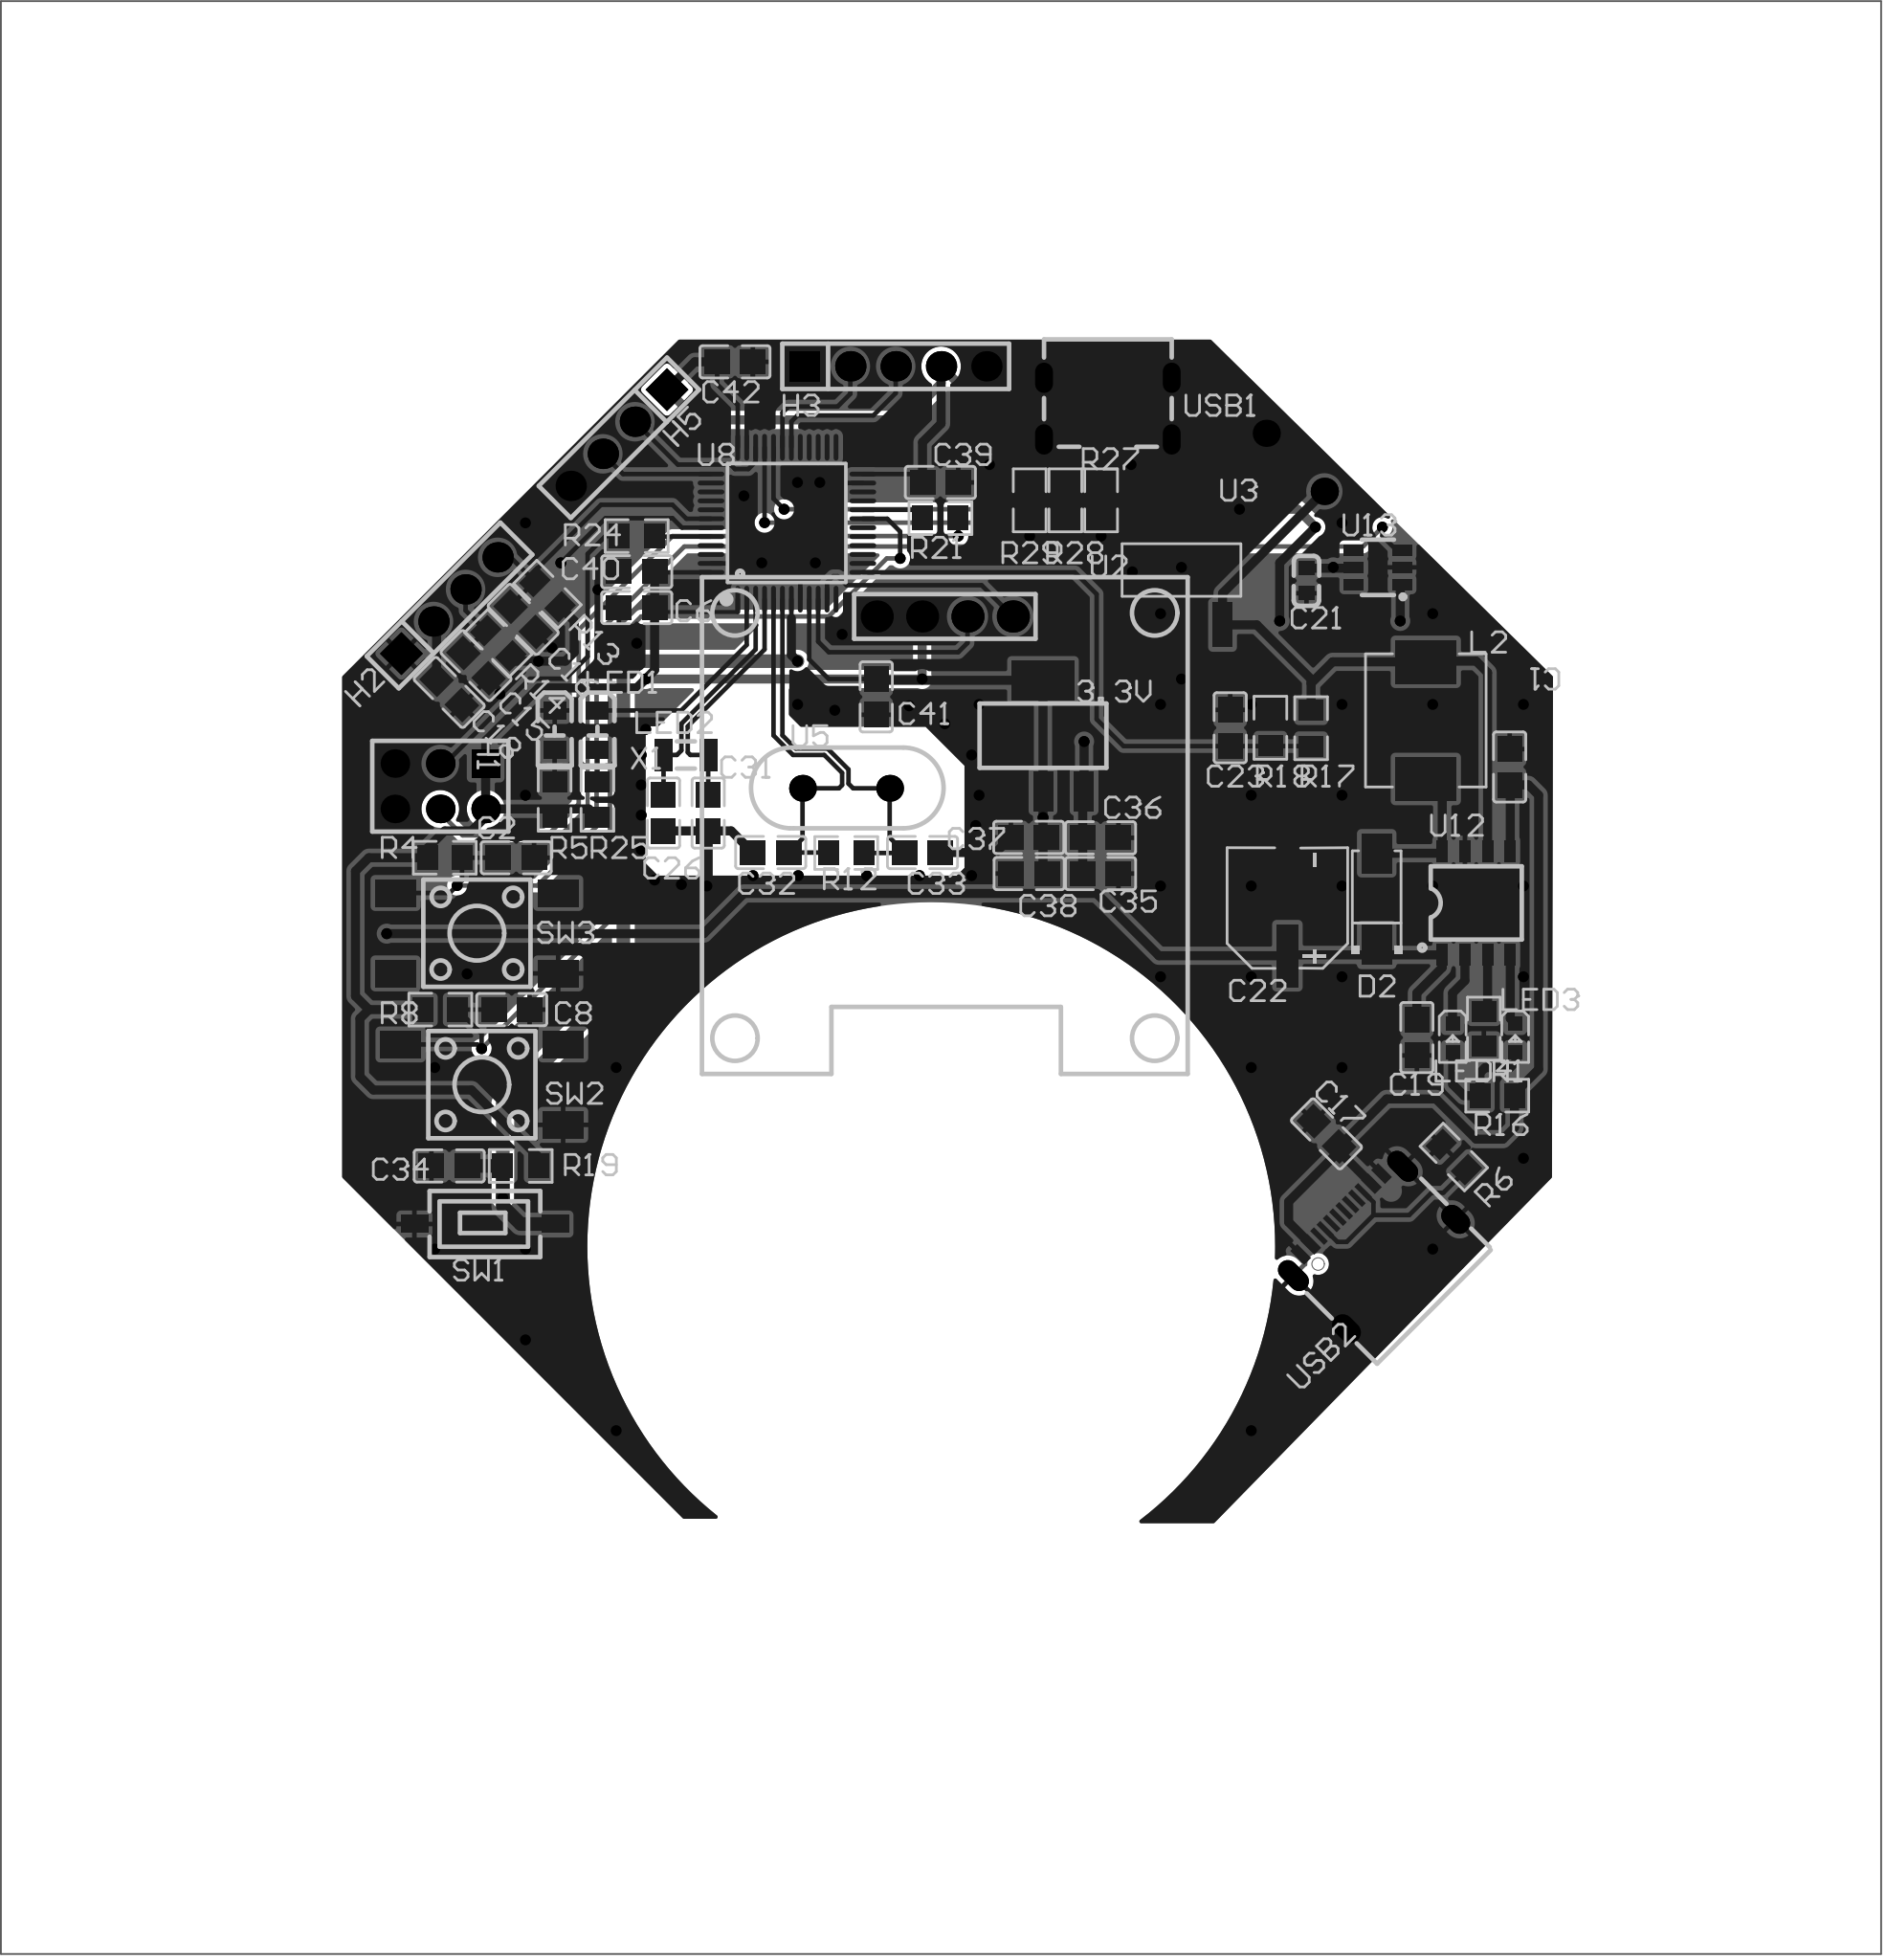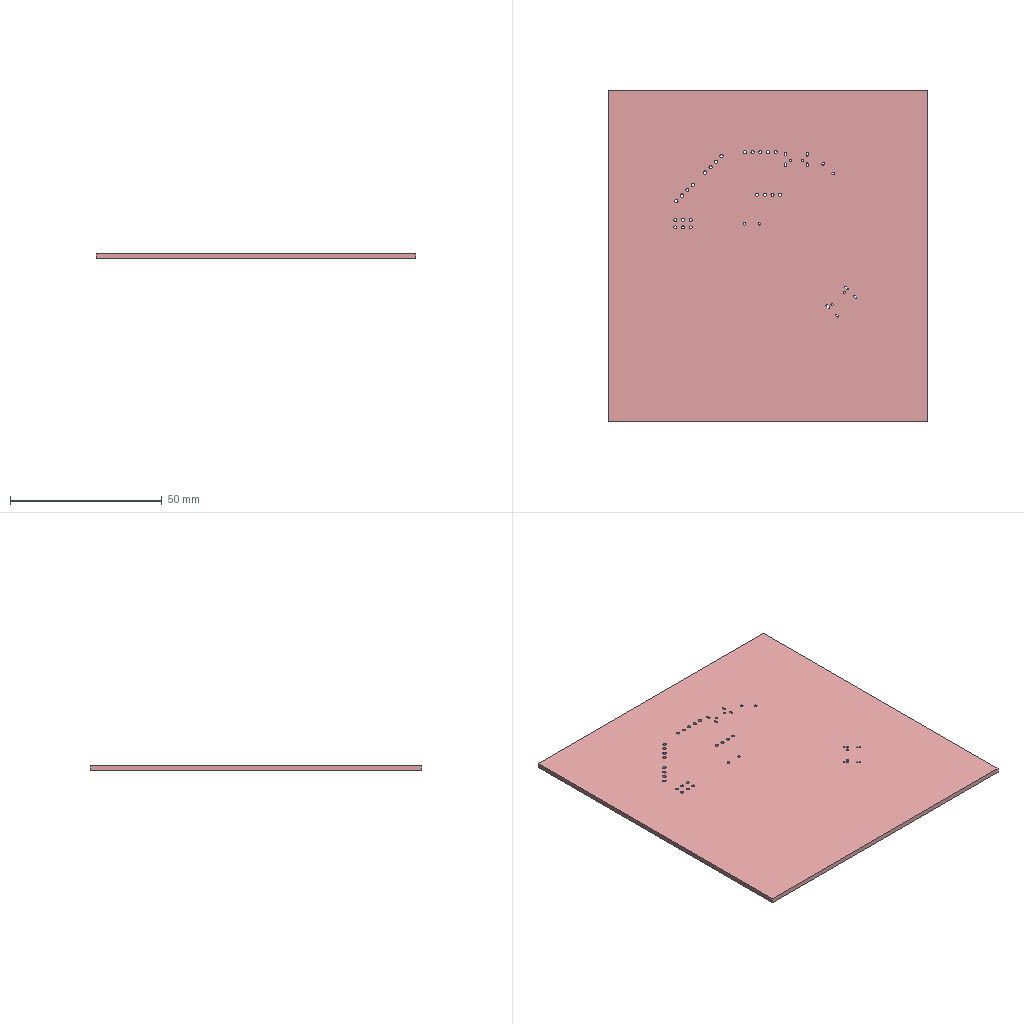Circuit board layout | Altium Designer | box 105.3 x 109.3 x 1.6 mm
Layer stack:
# Altium Designer layer stack of  (unit mm; dielectric type: 0 none, 1 core, 2 prepreg, 3 surface material)
index,name,kind,layer,copper_thickness_mm,dielectric_type,dielectric_thickness_mm,dielectric_material,dielectric_constant
0,Top Paste Mask Layer,other,,,,,,
1,Top Silkscreen Layer,other,,,,,,
2,Top Solder Mask Layer,dielectric,,,3,0.01,,3.3
3,Top Layer,copper,Top Layer,0.035,,,,
4,Dielectric1,dielectric,,,3,1.51,FR4,4.5
5,Bottom Layer,copper,Bottom Layer,0.035,,,,
6,Bottom Solder Mask Layer,dielectric,,,3,0.01,,3.3
7,Bottom Silkscreen Layer,other,,,,,,
8,Bottom Paste Mask Layer,other,,,,,,
# drill layer pairs: low layer,high layer
drill_pair,Top Layer,Bottom Layer
Part placement:
Designator,Comment,Layer,Footprint,Center-X(mm),Center-Y(mm),Rotation
R1,10Ω,TopLayer,R0805_NEW,152.883,121.634,90
C2,0.1uF,TopLayer,C0805,98.703,131.2,0
R12,1M,TopLayer,R0805,117.181,131.464,180
USB1,,TopLayer,USB_Micro,131.832,156.333,180
C8,0.1uF,TopLayer,C0805,98.453,122.7,0
C37,10UF,TopLayer,C0805,127.401,132.338,0
R21,10K,TopLayer,R0805,122.457,150.2,180
R25,510R,TopLayer,R0805,103.252,134.445,90
R28,20R,TopLayer,R0805,129.452,151.2,270
C38,100nF,TopLayer,C0805,127.422,130.314,0
C39,100nF,TopLayer,C0805,122.453,152.2,180
C15,0.1uF,TopLayer,C0805,96.453,141.95,135
C40,100nF,TopLayer,C0805,105.453,147.2,0
C16,0.1uF,TopLayer,C0805,99.095,144.539,135
C17,0.1uF,TopLayer,C0805,144.07,115.746,315
C18,0.1uF,TopLayer,C0805,94.953,140.45,315
C41,100nF,TopLayer,C0805,118.861,140.2,90
C19,100nF,TopLayer,C0805,149.133,121.134,270
C42,100nF,TopLayer,C0805,110.953,158.95,180
C21,100nF,TopLayer,C0603,142.952,146.7,90
C1,10uF,TopLayer,C0805,154.329,136.277,270
C22,47uF,TopLayer,CAP-SMD_BD6.3-L6.6-W6.6-LS7.2-FD,141.884,128.384,90
C23,100nF,TopLayer,C0805,138.681,138.471,90
H1,,TopLayer,HDR-TH_6P-P2.54-V-R2-C3-S2.54_A2541WV-2X3P,94.453,135.2,180
D2,SS14,TopLayer,SMA_L4.2-W2.6-LS5.3-RD,146.883,128.884,90
R19,10K,TopLayer,R0805,98.953,113.95,0
H2,2.54-1*4P排针母座,TopLayer,HDR-TH_4P-P2.54-V-F,94.97,145.316,45
H3,PZ254-1-05-Z-8.5,TopLayer,HDR-TH_5P-P2.54-V-M,119.953,158.7,0
R27,20R,TopLayer,R0805,131.452,151.2,270
SW1,,TopLayer,Key_SMD_3.6x6.1x2.5,96.953,110.7,0
L2,10uH,TopLayer,IND-SMD_L7.3-W6.6,149.633,138.884,270
C32,20PF,TopLayer,C0805,112.953,131.489,180
C33,20PF,TopLayer,C0805,121.453,131.489,0
U5,8MHz,TopLayer,CRYSTAL-TH_L10.8-W4.5-P4.88,117.174,135.085,180
R4,10K,TopLayer,R0805_NEW,94.703,131.2,180
R6,5.1kΩ,TopLayer,R0805,151.202,114.45,135
LED2,,TopLayer,LED_0805,103.257,138.341,270
R8,10K,TopLayer,R0805_NEW,94.453,122.7,180
C6,100nF,TopLayer,C0805,105.453,145.2,0
3.3V,,TopLayer,SOT_223,128.201,138.029,0
C36,100nF,TopLayer,C0805,131.423,132.314,180
R5,510R,TopLayer,R0805,100.853,134.445,90
R13,1kΩ,TopLayer,R0805,100.453,145.95,315
C35,1UF,TopLayer,C0805,131.423,130.314,180
R14,1kΩ,TopLayer,R0805,97.703,143.2,315
C31,20PF,TopLayer,C0805,109.453,133.7,90
R16,2K,TopLayer,R0805_NEW,153.633,117.884,0
LED3,NCD0603R1,TopLayer,LED0603-RD_RED,154.633,121.134,270
R17,100kΩ,TopLayer,R0805,143.21,138.446,270
LED4,NCD0603R1,TopLayer,LED0603-RD_RED,151.133,121.134,270
R18,100kΩ,TopLayer,R0805,140.931,138.471,90
SW2,TS-1002S-13026C,TopLayer,SW-SMD_4P-L6.0-W6.0-P4.50-LS9.0-2,96.78,118.5,0
SW3,TS-1002S-13026C,TopLayer,SW-SMD_4P-L6.0-W6.0-P4.50-LS9.0-2,96.503,126.976,0
LED1,,TopLayer,LED_0805,100.858,138.341,270
H5,,TopLayer,HDR-TH_4P-P2.54-V-M,104.453,154.7,225
R29,5.1K,TopLayer,R0805,127.453,151.2,270
U3,AMS1117-3.3,TopLayer,SOT-223-3_L6.5-W3.5-P3.05-LS7.0,135.952,147.2,270
R24,10K,TopLayer,R0805,105.448,149.2,180
C34,105,0603,TopLayer,C0805,94.953,113.95,0
U8,STM32F103C8T6,TopLayer,LQFP-48_L7.0-W7.0-P0.50-LS9.0-BL,113.86,149.919,0
USB2,TYPE-C 16PIN 2MD(073),TopLayer,USB-C-SMD_TYPE-C-6PIN-2MD-073,146.765,109.388,45
X1,32.768kHz,TopLayer,FC-135R_L3.2-W1.5,108.203,136.95,180
U12,TP5400,TopLayer,ESOP-8_L4.9-W3.9-P1.27-LS6.0-BL-EP,152.459,128.669,0
C26,20PF,TopLayer,C0805,106.953,133.7,270
U13,EC190708,TopLayer,SOT-23-6_L2.9-W1.6-P0.95-LS2.8-BR,146.952,147.45,0
U2,HS96L03W2C03,TopLayer,OLED-TH_L27.8-W27.2-P2.54_C9900033791,122.703,144.7,0
Pad and via stacks:
# Altium Designer via and pad stacks of  (unit mm). Each distinct definition once, with the count of objects using it.
# via: kind,start_layer,end_layer,hole_mm,diameter_mm,mode(0 simple;1 top-mid-bottom;2 full stack),diameter_per_layer,count,example_net
# pad: kind,layer,hole_mm,hole_type(0 round;1 square;2 slot),plating,top_size,top_shape(1 round;2 rect;3 octagon;9 rounded rect),mid_size,bottom_size,mode,footprint,size_per_layer,count,example
pad,Multi-Layer,0.9144,0,plated,1.524x1.524,1,1.524x1.524,1.524x1.524,0,,,2,1
pad,Multi-Layer,0.6,2,plated,1x1.7,1,1x1.7,1x1.7,0,USB_Micro,,4,USB1.6
pad,Multi-Layer,1.05,0,plated,1.6x1.6,2,1.6x1.6,1.6x1.6,0,HDR-TH_6P-P2.54-V-R2-C3-S2.54_A2541WV-2X3P,,1,H1.1
pad,Multi-Layer,1.05,0,plated,1.6x1.6,1,1.6x1.6,1.6x1.6,0,HDR-TH_6P-P2.54-V-R2-C3-S2.54_A2541WV-2X3P,,5,H1.2
pad,Multi-Layer,1.1,0,plated,1.7x1.7,2,1.7x1.7,1.7x1.7,0,HDR-TH_4P-P2.54-V-F,,1,H2.1
pad,Multi-Layer,1.1,0,plated,1.7x1.7,1,1.7x1.7,1.7x1.7,0,HDR-TH_4P-P2.54-V-F,,3,H2.2
pad,Multi-Layer,1.1,0,plated,1.7x1.7,2,1.7x1.7,1.7x1.7,0,HDR-TH_5P-P2.54-V-M,,1,H3.1
pad,Multi-Layer,1.1,0,plated,1.7x1.7,1,1.7x1.7,1.7x1.7,0,HDR-TH_5P-P2.54-V-M,,4,H3.2
pad,Multi-Layer,0.8,0,plated,1.5x1.5,1,1.5x1.5,1.5x1.5,0,CRYSTAL-TH_L10.8-W4.5-P4.88,,2,U5.1
pad,Multi-Layer,1.1,0,plated,1.7x1.7,2,1.7x1.7,1.7x1.7,0,HDR-TH_4P-P2.54-V-M,,1,H5.1
pad,Multi-Layer,1.1,0,plated,1.7x1.7,1,1.7x1.7,1.7x1.7,0,HDR-TH_4P-P2.54-V-M,,3,H5.2
pad,Multi-Layer,0.6,2,plated,1.1x2,1,1.1x2,1.1x2,0,USB-C-SMD_TYPE-C-6PIN-2MD-073,,2,USB2.13
pad,Multi-Layer,0.6,2,plated,1.2x1.8,1,1.2x1.8,1.2x1.8,0,USB-C-SMD_TYPE-C-6PIN-2MD-073,,2,USB2.13
pad,Multi-Layer,1.05,0,plated,1.8x1.8,1,1.8x1.8,1.8x1.8,0,OLED-TH_L27.8-W27.2-P2.54_C9900033791,,4,U2.1
pad,Top Layer,0,0,plated,1.133x1.377,2,1.133x1.377,1.133x1.377,0,R0805_NEW,,8,R1.2
pad,Top Layer,0,0,plated,1.41x1.35,2,1.41x1.35,1.41x1.35,0,C0805,,46,C2.2
pad,Top Layer,0,0,plated,1.133x1.377,2,1.133x1.377,1.133x1.377,0,R0805,,28,R12.2
pad,Top Layer,0,0,plated,0.4x1.4,2,0.4x1.4,0.4x1.4,0,USB_Micro,,5,USB1.1
pad,Top Layer,0,0,plated,0.8x0.9,2,0.8x0.9,0.8x0.9,0,C0603,,2,C21.2
pad,Top Layer,0,0,plated,3.5x1.2,2,3.5x1.2,3.5x1.2,0,CAP-SMD_BD6.3-L6.6-W6.6-LS7.2-FD,,2,C22.2
pad,Top Layer,0,0,plated,2.2x1.7,2,2.2x1.7,2.2x1.7,0,SMA_L4.2-W2.6-LS5.3-RD,,2,D2.1
pad,Top Layer,0,0,plated,1.501x1.001,2,1.501x1.001,1.501x1.001,0,Key_SMD_3.6x6.1x2.5,,2,SW1.2
pad,Top Layer,0,0,plated,2.424x3.42,2,2.424x3.42,2.424x3.42,0,IND-SMD_L7.3-W6.6,,2,L2.1
pad,Top Layer,0,0,plated,1x1.25,2,1x1.25,1x1.25,0,LED_0805,,4,LED2.2
pad,Top Layer,0,0,plated,2.2x3.5,2,2.2x3.5,2.2x3.5,0,SOT_223,,1,3.3V.4
pad,Top Layer,0,0,plated,1.1x2.2,2,1.1x2.2,1.1x2.2,0,SOT_223,,3,3.3V.3
pad,Top Layer,0,0,plated,0.8x0.8,2,0.8x0.8,0.8x0.8,0,LED0603-RD_RED,,4,LED3.1
pad,Top Layer,0,0,plated,2.3x1.5,2,2.3x1.5,2.3x1.5,0,SW-SMD_4P-L6.0-W6.0-P4.50-LS9.0-2,,8,SW2.1
pad,Top Layer,0,0,plated,2.34x3.6,2,2.34x3.6,2.34x3.6,0,SOT-223-3_L6.5-W3.5-P3.05-LS7.0,,1,U3.4
pad,Top Layer,0,0,plated,2.5x1.1,2,2.5x1.1,2.5x1.1,0,SOT-223-3_L6.5-W3.5-P3.05-LS7.0,,3,U3.3
pad,Top Layer,0,0,plated,0.27x1.5,1,0.27x1.5,0.27x1.5,0,LQFP-48_L7.0-W7.0-P0.50-LS9.0-BL,,24,U8.1
pad,Top Layer,0,0,plated,1.5x0.27,1,1.5x0.27,1.5x0.27,0,LQFP-48_L7.0-W7.0-P0.50-LS9.0-BL,,24,U8.13
pad,Top Layer,0,0,plated,0.55x1.1,2,0.55x1.1,0.55x1.1,0,USB-C-SMD_TYPE-C-6PIN-2MD-073,,4,USB2.1
pad,Top Layer,0,0,plated,0.3x1.1,2,0.3x1.1,0.3x1.1,0,USB-C-SMD_TYPE-C-6PIN-2MD-073,,8,USB2.3
pad,Top Layer,0,0,plated,1.8x1,2,1.8x1,1.8x1,0,FC-135R_L3.2-W1.5,,2,X1.1
pad,Top Layer,0,0,plated,0.6x1.2,2,0.6x1.2,0.6x1.2,0,ESOP-8_L4.9-W3.9-P1.27-LS6.0-BL-EP,,8,U12.1
pad,Top Layer,0,0,plated,3.3x2.4,2,3.3x2.4,3.3x2.4,0,ESOP-8_L4.9-W3.9-P1.27-LS6.0-BL-EP,,1,U12.9
pad,Top Layer,0,0,plated,1.1x0.6,2,1.1x0.6,1.1x0.6,0,SOT-23-6_L2.9-W1.6-P0.95-LS2.8-BR,,6,U13.3
via,Top Layer,Bottom Layer,0.3048,0.61,0,,92,$2N3585
Copper pours:
name,layer,net,type(0 solid;1 hatched;2 none)
Top Layer-GND,Top Layer,GND,0
Bottom Layer-GND,Bottom Layer,GND,0
Design rules, without the lines most boards share:
# Altium Designer design rules of  (exported by Altium Designer, unit mm)
# columns: name | kind | enabled | priority | scope1 | scope2 | descriptor | typed fields (field=value)
copperThicknessInner0.5oz | 0 | disabled | 2 | All | All | Clearance Constraint (Gap=5.984mil) (Disabled)(All),(All) | gap=0.152
copperThicknessInner0.5oz_1 | 63 | disabled | 2 | All | All | Board Clearance Constraint (Gap=0mil) (Disabled)(All) |
Plane_innerPlane | 0 | disabled | 3 | All | All | Clearance Constraint (Gap=5.984mil) (Disabled)(All),(All) | gap=0.152
Plane_innerPlane_1 | 63 | disabled | 3 | All | All | Board Clearance Constraint (Gap=0mil) (Disabled)(All) |
Copper_copperRegion | 0 | disabled | 4 | All | All | Clearance Constraint (Gap=5.984mil) (Disabled)(All),(All) | gap=0.152
Copper_copperRegion_1 | 63 | disabled | 4 | All | All | Board Clearance Constraint (Gap=0mil) (Disabled)(All) |
Copper_copperRegion1 | 0 | disabled | 5 | All | All | Clearance Constraint (Gap=5.984mil) (Disabled)(All),(All) | gap=0.152
Copper_copperRegion1_1 | 63 | disabled | 5 | All | All | Board Clearance Constraint (Gap=0mil) (Disabled)(All) |
copperThickness1oz | 0 | enabled | 6 | All | All | Clearance Constraint (Gap=5.984mil) (All),(All) | gap=0.152
copperThickness1oz_1 | 63 | enabled | 6 | All | All | Board Clearance Constraint (Gap=0mil) (All) |
otherClearance | 52 | enabled | 1 | All | All | Hole To Hole Clearance (Gap=11.8mil) (All),(All) | gap=0.2997
copperThickness0.5oz | 2 | disabled | 2 | All | All | Width Constraint (Min=3.5mil) (Max=100mil) (Preferred=10mil) (Disabled)(All) |
copperThickness1oz_2 | 2 | enabled | 3 | All | All | Width Constraint (Min=4mil) (Max=100mil) (Preferred=10mil) (All) |
copperRegion1 | 20 | disabled | 1 | All | All | Polygon Connect Rule(Relief Connect )(Conductor Width=10mil) (Relief Angle=90 Angle) (Entries=4) (Air Gap Width=10mil) (Disabled)(All),(All) | connect_style(0=relief,1=direct,2=none)=0 relief_conductor_width=0.254 relief_entries=4
copperRegion | 20 | enabled | 2 | All | All | Polygon Connect Rule(Relief Connect )(Conductor Width=10mil) (Relief Angle=90 Angle) (Entries=4) (Air Gap Width=10mil) (All),(All) | connect_style(0=relief,1=direct,2=none)=0 relief_conductor_width=0.254 relief_entries=4
solderMaskExpansion | 13 | enabled | 2 | All | All | Solder Mask Expansion (Expansion =2.008mil) (All) | expansion=0.051